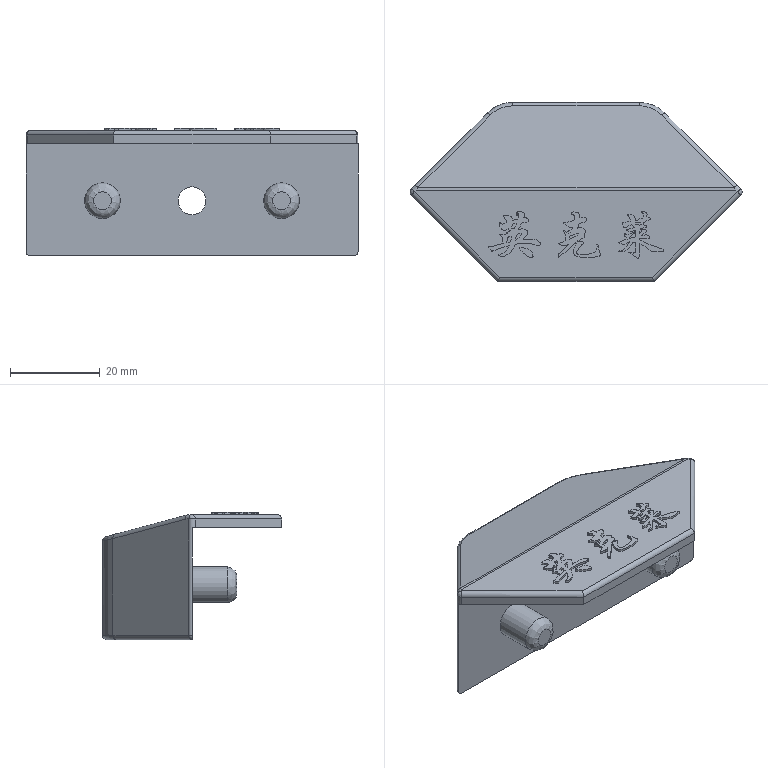Part | STEP file | DECH07 | 1 solid | 206 faces | box 74.172 x 40 x 28.5 mm | volume 30644 mm3 | spline 146 | plane 32 | cylinder 18 | sphere 4 | torus 3 | other 2 | cone 1 | commonest cylinder face diameters 2 x11 8 x2 16 x2 5 x1 6.2 x1 12 x1